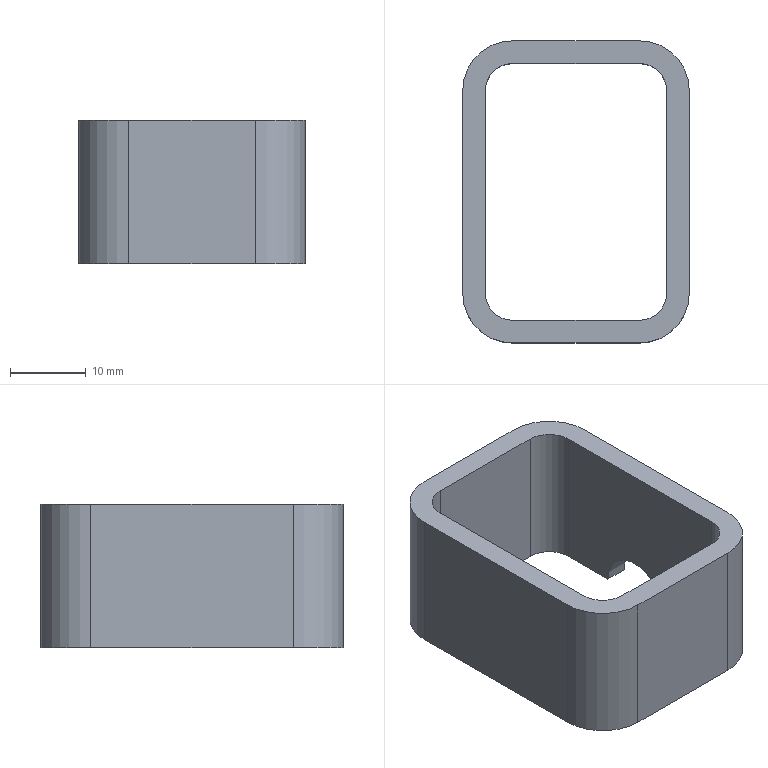Part | STEP file | DIN EN 10305-5 40 x 30 x 3 1785420022083 | 1 solid | 19 faces | box 30 x 40 x 19 mm | volume 6679 mm3 | plane 10 | cylinder 9 | commonest cylinder face diameters 7.2 x4 13.2 x4 10 x1
STEP:
#1=CARTESIAN_POINT('',(15.,-13.4,19.));
#2=VERTEX_POINT('',#1);
#3=CARTESIAN_POINT('',(8.4,-20.,19.));
#4=VERTEX_POINT('',#3);
#5=CARTESIAN_POINT('',(8.4,-13.4,19.));
#6=DIRECTION('',(0.,0.,-1.));
#7=DIRECTION('',(0.,1.,0.));
#8=AXIS2_PLACEMENT_3D('',#5,#6,#7);
#9=CIRCLE('',#8,6.6);
#10=EDGE_CURVE('',#2,#4,#9,.T.);
#11=ORIENTED_EDGE('',*,*,#10,.F.);
#12=CARTESIAN_POINT('',(15.,13.4,19.));
#13=VERTEX_POINT('',#12);
#14=CARTESIAN_POINT('',(15.,-48.3,19.));
#15=DIRECTION('',(0.,-1.,0.));
#16=VECTOR('',#15,10.);
#17=LINE('',#14,#16);
#18=EDGE_CURVE('',#13,#2,#17,.T.);
#19=ORIENTED_EDGE('',*,*,#18,.F.);
#20=CARTESIAN_POINT('',(8.4,20.,19.));
#21=VERTEX_POINT('',#20);
#22=CARTESIAN_POINT('',(8.4,13.4,19.));
#23=DIRECTION('',(0.,0.,-1.));
#24=DIRECTION('',(-1.,0.,0.));
#25=AXIS2_PLACEMENT_3D('',#22,#23,#24);
#26=CIRCLE('',#25,6.6);
#27=EDGE_CURVE('',#21,#13,#26,.T.);
#28=ORIENTED_EDGE('',*,*,#27,.F.);
#29=CARTESIAN_POINT('',(-8.4,20.,19.));
#30=VERTEX_POINT('',#29);
#31=CARTESIAN_POINT('',(-4.2,20.,19.));
#32=DIRECTION('',(1.,0.,0.));
#33=VECTOR('',#32,10.);
#34=LINE('',#31,#33);
#35=EDGE_CURVE('',#30,#21,#34,.T.);
#36=ORIENTED_EDGE('',*,*,#35,.F.);
#37=CARTESIAN_POINT('',(-15.,13.4,19.));
#38=VERTEX_POINT('',#37);
#39=CARTESIAN_POINT('',(-8.4,13.4,19.));
#40=DIRECTION('',(0.,0.,-1.));
#41=DIRECTION('',(0.,-1.,0.));
#42=AXIS2_PLACEMENT_3D('',#39,#40,#41);
#43=CIRCLE('',#42,6.6);
#44=EDGE_CURVE('',#38,#30,#43,.T.);
#45=ORIENTED_EDGE('',*,*,#44,.F.);
#46=CARTESIAN_POINT('',(-15.,-13.4,19.));
#47=VERTEX_POINT('',#46);
#48=CARTESIAN_POINT('',(-15.,-61.7,19.));
#49=DIRECTION('',(0.,1.,0.));
#50=VECTOR('',#49,10.);
#51=LINE('',#48,#50);
#52=EDGE_CURVE('',#47,#38,#51,.T.);
#53=ORIENTED_EDGE('',*,*,#52,.F.);
#54=CARTESIAN_POINT('',(-8.4,-20.,19.));
#55=VERTEX_POINT('',#54);
#56=CARTESIAN_POINT('',(-8.4,-13.4,19.));
#57=DIRECTION('',(0.,0.,-1.));
#58=DIRECTION('',(1.,0.,0.));
#59=AXIS2_PLACEMENT_3D('',#56,#57,#58);
#60=CIRCLE('',#59,6.6);
#61=EDGE_CURVE('',#55,#47,#60,.T.);
#62=ORIENTED_EDGE('',*,*,#61,.F.);
#63=CARTESIAN_POINT('',(4.2,-20.,19.));
#64=DIRECTION('',(-1.,0.,0.));
#65=VECTOR('',#64,10.);
#66=LINE('',#63,#65);
#67=EDGE_CURVE('',#4,#55,#66,.T.);
#68=ORIENTED_EDGE('',*,*,#67,.F.);
#69=EDGE_LOOP('',(#11,#19,#28,#36,#45,#53,#62,#68));
#70=FACE_OUTER_BOUND('',#69,.T.);
#71=CARTESIAN_POINT('',(12.,-13.4,19.));
#72=VERTEX_POINT('',#71);
#73=CARTESIAN_POINT('',(12.,13.4,19.));
#74=VERTEX_POINT('',#73);
#75=CARTESIAN_POINT('',(12.,-48.3,19.));
#76=DIRECTION('',(0.,1.,0.));
#77=VECTOR('',#76,10.);
#78=LINE('',#75,#77);
#79=EDGE_CURVE('',#72,#74,#78,.T.);
#80=ORIENTED_EDGE('',*,*,#79,.F.);
#81=CARTESIAN_POINT('',(8.4,-17.,19.));
#82=VERTEX_POINT('',#81);
#83=CARTESIAN_POINT('',(8.4,-13.4,19.));
#84=DIRECTION('',(0.,0.,1.));
#85=DIRECTION('',(0.,1.,0.));
#86=AXIS2_PLACEMENT_3D('',#83,#84,#85);
#87=CIRCLE('',#86,3.6);
#88=EDGE_CURVE('',#82,#72,#87,.T.);
#89=ORIENTED_EDGE('',*,*,#88,.F.);
#90=CARTESIAN_POINT('',(-8.4,-17.,19.));
#91=VERTEX_POINT('',#90);
#92=CARTESIAN_POINT('',(4.2,-17.,19.));
#93=DIRECTION('',(1.,0.,0.));
#94=VECTOR('',#93,10.);
#95=LINE('',#92,#94);
#96=EDGE_CURVE('',#91,#82,#95,.T.);
#97=ORIENTED_EDGE('',*,*,#96,.F.);
#98=CARTESIAN_POINT('',(-12.,-13.4,19.));
#99=VERTEX_POINT('',#98);
#100=CARTESIAN_POINT('',(-8.4,-13.4,19.));
#101=DIRECTION('',(0.,0.,1.));
#102=DIRECTION('',(1.,0.,0.));
#103=AXIS2_PLACEMENT_3D('',#100,#101,#102);
#104=CIRCLE('',#103,3.6);
#105=EDGE_CURVE('',#99,#91,#104,.T.);
#106=ORIENTED_EDGE('',*,*,#105,.F.);
#107=CARTESIAN_POINT('',(-12.,13.4,19.));
#108=VERTEX_POINT('',#107);
#109=CARTESIAN_POINT('',(-12.,-61.7,19.));
#110=DIRECTION('',(0.,-1.,0.));
#111=VECTOR('',#110,10.);
#112=LINE('',#109,#111);
#113=EDGE_CURVE('',#108,#99,#112,.T.);
#114=ORIENTED_EDGE('',*,*,#113,.F.);
#115=CARTESIAN_POINT('',(-8.4,17.,19.));
#116=VERTEX_POINT('',#115);
#117=CARTESIAN_POINT('',(-8.4,13.4,19.));
#118=DIRECTION('',(0.,0.,1.));
#119=DIRECTION('',(0.,-1.,0.));
#120=AXIS2_PLACEMENT_3D('',#117,#118,#119);
#121=CIRCLE('',#120,3.6);
#122=EDGE_CURVE('',#116,#108,#121,.T.);
#123=ORIENTED_EDGE('',*,*,#122,.F.);
#124=CARTESIAN_POINT('',(8.4,17.,19.));
#125=VERTEX_POINT('',#124);
#126=CARTESIAN_POINT('',(-4.2,17.,19.));
#127=DIRECTION('',(-1.,0.,0.));
#128=VECTOR('',#127,10.);
#129=LINE('',#126,#128);
#130=EDGE_CURVE('',#125,#116,#129,.T.);
#131=ORIENTED_EDGE('',*,*,#130,.F.);
#132=CARTESIAN_POINT('',(8.4,13.4,19.));
#133=DIRECTION('',(0.,0.,1.));
#134=DIRECTION('',(-1.,0.,0.));
#135=AXIS2_PLACEMENT_3D('',#132,#133,#134);
#136=CIRCLE('',#135,3.6);
#137=EDGE_CURVE('',#74,#125,#136,.T.);
#138=ORIENTED_EDGE('',*,*,#137,.F.);
#139=EDGE_LOOP('',(#80,#89,#97,#106,#114,#123,#131,#138));
#140=FACE_BOUND('',#139,.T.);
#141=CARTESIAN_POINT('',(0.,-110.,19.));
#142=DIRECTION('',(0.,0.,1.));
#143=DIRECTION('',(-1.,0.,0.));
#144=AXIS2_PLACEMENT_3D('',#141,#142,#143);
#145=PLANE('',#144);
#146=ADVANCED_FACE('',(#70,#140),#145,.T.);
#147=ORIENTED_EDGE('',*,*,#137,.T.);
#148=CARTESIAN_POINT('',(8.4,17.,0.));
#149=VERTEX_POINT('',#148);
#150=CARTESIAN_POINT('',(8.4,17.,0.));
#151=DIRECTION('',(0.,0.,1.));
#152=VECTOR('',#151,10.);
#153=LINE('',#150,#152);
#154=EDGE_CURVE('',#149,#125,#153,.T.);
#155=ORIENTED_EDGE('',*,*,#154,.F.);
#156=CARTESIAN_POINT('',(12.,13.4,0.));
#157=VERTEX_POINT('',#156);
#158=CARTESIAN_POINT('',(8.4,13.4,0.));
#159=DIRECTION('',(0.,0.,1.));
#160=DIRECTION('',(-1.,0.,0.));
#161=AXIS2_PLACEMENT_3D('',#158,#159,#160);
#162=CIRCLE('',#161,3.6);
#163=EDGE_CURVE('',#157,#149,#162,.T.);
#164=ORIENTED_EDGE('',*,*,#163,.F.);
#165=CARTESIAN_POINT('',(12.,13.4,0.));
#166=DIRECTION('',(0.,0.,1.));
#167=VECTOR('',#166,10.);
#168=LINE('',#165,#167);
#169=EDGE_CURVE('',#157,#74,#168,.T.);
#170=ORIENTED_EDGE('',*,*,#169,.T.);
#171=EDGE_LOOP('',(#147,#155,#164,#170));
#172=FACE_OUTER_BOUND('',#171,.T.);
#173=CARTESIAN_POINT('',(8.4,13.4,0.));
#174=DIRECTION('',(0.,0.,1.));
#175=DIRECTION('',(-1.,0.,0.));
#176=AXIS2_PLACEMENT_3D('',#173,#174,#175);
#177=CYLINDRICAL_SURFACE('',#176,3.6);
#178=ADVANCED_FACE('',(#172),#177,.F.);
#179=ORIENTED_EDGE('',*,*,#130,.T.);
#180=CARTESIAN_POINT('',(-8.4,17.,0.));
#181=VERTEX_POINT('',#180);
#182=CARTESIAN_POINT('',(-8.4,17.,0.));
#183=DIRECTION('',(0.,0.,1.));
#184=VECTOR('',#183,10.);
#185=LINE('',#182,#184);
#186=EDGE_CURVE('',#181,#116,#185,.T.);
#187=ORIENTED_EDGE('',*,*,#186,.F.);
#188=CARTESIAN_POINT('',(-4.2,17.,0.));
#189=DIRECTION('',(-1.,0.,0.));
#190=VECTOR('',#189,10.);
#191=LINE('',#188,#190);
#192=EDGE_CURVE('',#149,#181,#191,.T.);
#193=ORIENTED_EDGE('',*,*,#192,.F.);
#194=ORIENTED_EDGE('',*,*,#154,.T.);
#195=EDGE_LOOP('',(#179,#187,#193,#194));
#196=FACE_OUTER_BOUND('',#195,.T.);
#197=CARTESIAN_POINT('',(-8.4,17.,0.));
#198=DIRECTION('',(0.,1.,0.));
#199=DIRECTION('',(0.,0.,1.));
#200=AXIS2_PLACEMENT_3D('',#197,#198,#199);
#201=PLANE('',#200);
#202=ADVANCED_FACE('',(#196),#201,.F.);
#203=ORIENTED_EDGE('',*,*,#122,.T.);
#204=CARTESIAN_POINT('',(-12.,13.4,0.));
#205=VERTEX_POINT('',#204);
#206=CARTESIAN_POINT('',(-12.,13.4,0.));
#207=DIRECTION('',(0.,0.,1.));
#208=VECTOR('',#207,10.);
#209=LINE('',#206,#208);
#210=EDGE_CURVE('',#205,#108,#209,.T.);
#211=ORIENTED_EDGE('',*,*,#210,.F.);
#212=CARTESIAN_POINT('',(-8.4,13.4,0.));
#213=DIRECTION('',(0.,0.,1.));
#214=DIRECTION('',(0.,-1.,0.));
#215=AXIS2_PLACEMENT_3D('',#212,#213,#214);
#216=CIRCLE('',#215,3.6);
#217=EDGE_CURVE('',#181,#205,#216,.T.);
#218=ORIENTED_EDGE('',*,*,#217,.F.);
#219=ORIENTED_EDGE('',*,*,#186,.T.);
#220=EDGE_LOOP('',(#203,#211,#218,#219));
#221=FACE_OUTER_BOUND('',#220,.T.);
#222=CARTESIAN_POINT('',(-8.4,13.4,0.));
#223=DIRECTION('',(0.,0.,1.));
#224=DIRECTION('',(0.,-1.,0.));
#225=AXIS2_PLACEMENT_3D('',#222,#223,#224);
#226=CYLINDRICAL_SURFACE('',#225,3.6);
#227=ADVANCED_FACE('',(#221),#226,.F.);
#228=ORIENTED_EDGE('',*,*,#113,.T.);
#229=CARTESIAN_POINT('',(-12.,-13.4,0.));
#230=VERTEX_POINT('',#229);
#231=CARTESIAN_POINT('',(-12.,-13.4,0.));
#232=DIRECTION('',(0.,0.,1.));
#233=VECTOR('',#232,10.);
#234=LINE('',#231,#233);
#235=EDGE_CURVE('',#230,#99,#234,.T.);
#236=ORIENTED_EDGE('',*,*,#235,.F.);
#237=CARTESIAN_POINT('',(-12.,-6.7,0.));
#238=DIRECTION('',(0.,-1.,0.));
#239=VECTOR('',#238,10.);
#240=LINE('',#237,#239);
#241=EDGE_CURVE('',#205,#230,#240,.T.);
#242=ORIENTED_EDGE('',*,*,#241,.F.);
#243=ORIENTED_EDGE('',*,*,#210,.T.);
#244=EDGE_LOOP('',(#228,#236,#242,#243));
#245=FACE_OUTER_BOUND('',#244,.T.);
#246=CARTESIAN_POINT('',(-12.,-13.4,0.));
#247=DIRECTION('',(-1.,0.,0.));
#248=DIRECTION('',(0.,0.,1.));
#249=AXIS2_PLACEMENT_3D('',#246,#247,#248);
#250=PLANE('',#249);
#251=ADVANCED_FACE('',(#245),#250,.F.);
#252=ORIENTED_EDGE('',*,*,#67,.T.);
#253=CARTESIAN_POINT('',(-8.4,-20.,0.));
#254=VERTEX_POINT('',#253);
#255=CARTESIAN_POINT('',(-8.4,-20.,0.));
#256=DIRECTION('',(0.,0.,1.));
#257=VECTOR('',#256,10.);
#258=LINE('',#255,#257);
#259=EDGE_CURVE('',#254,#55,#258,.T.);
#260=ORIENTED_EDGE('',*,*,#259,.F.);
#261=CARTESIAN_POINT('',(8.4,-20.,0.));
#262=VERTEX_POINT('',#261);
#263=CARTESIAN_POINT('',(4.2,-20.,0.));
#264=DIRECTION('',(-1.,0.,0.));
#265=VECTOR('',#264,10.);
#266=LINE('',#263,#265);
#267=EDGE_CURVE('',#262,#254,#266,.T.);
#268=ORIENTED_EDGE('',*,*,#267,.F.);
#269=CARTESIAN_POINT('',(8.4,-20.,0.));
#270=DIRECTION('',(0.,0.,1.));
#271=VECTOR('',#270,10.);
#272=LINE('',#269,#271);
#273=EDGE_CURVE('',#262,#4,#272,.T.);
#274=ORIENTED_EDGE('',*,*,#273,.T.);
#275=EDGE_LOOP('',(#252,#260,#268,#274));
#276=FACE_OUTER_BOUND('',#275,.T.);
#277=CARTESIAN_POINT('',(8.4,-20.,0.));
#278=DIRECTION('',(0.,-1.,0.));
#279=DIRECTION('',(0.,0.,-1.));
#280=AXIS2_PLACEMENT_3D('',#277,#278,#279);
#281=PLANE('',#280);
#282=ADVANCED_FACE('',(#276),#281,.T.);
#283=ORIENTED_EDGE('',*,*,#61,.T.);
#284=CARTESIAN_POINT('',(-15.,-13.4,0.));
#285=VERTEX_POINT('',#284);
#286=CARTESIAN_POINT('',(-15.,-13.4,0.));
#287=DIRECTION('',(0.,0.,1.));
#288=VECTOR('',#287,10.);
#289=LINE('',#286,#288);
#290=EDGE_CURVE('',#285,#47,#289,.T.);
#291=ORIENTED_EDGE('',*,*,#290,.F.);
#292=CARTESIAN_POINT('',(-8.4,-13.4,0.));
#293=DIRECTION('',(0.,0.,-1.));
#294=DIRECTION('',(1.,0.,0.));
#295=AXIS2_PLACEMENT_3D('',#292,#293,#294);
#296=CIRCLE('',#295,6.6);
#297=EDGE_CURVE('',#254,#285,#296,.T.);
#298=ORIENTED_EDGE('',*,*,#297,.F.);
#299=ORIENTED_EDGE('',*,*,#259,.T.);
#300=EDGE_LOOP('',(#283,#291,#298,#299));
#301=FACE_OUTER_BOUND('',#300,.T.);
#302=CARTESIAN_POINT('',(-8.4,-13.4,0.));
#303=DIRECTION('',(0.,0.,1.));
#304=DIRECTION('',(1.,0.,0.));
#305=AXIS2_PLACEMENT_3D('',#302,#303,#304);
#306=CYLINDRICAL_SURFACE('',#305,6.6);
#307=ADVANCED_FACE('',(#301),#306,.T.);
#308=ORIENTED_EDGE('',*,*,#52,.T.);
#309=CARTESIAN_POINT('',(-15.,13.4,0.));
#310=VERTEX_POINT('',#309);
#311=CARTESIAN_POINT('',(-15.,13.4,0.));
#312=DIRECTION('',(0.,0.,1.));
#313=VECTOR('',#312,10.);
#314=LINE('',#311,#313);
#315=EDGE_CURVE('',#310,#38,#314,.T.);
#316=ORIENTED_EDGE('',*,*,#315,.F.);
#317=CARTESIAN_POINT('',(-15.,-6.7,0.));
#318=DIRECTION('',(0.,1.,0.));
#319=VECTOR('',#318,10.);
#320=LINE('',#317,#319);
#321=EDGE_CURVE('',#285,#310,#320,.T.);
#322=ORIENTED_EDGE('',*,*,#321,.F.);
#323=ORIENTED_EDGE('',*,*,#290,.T.);
#324=EDGE_LOOP('',(#308,#316,#322,#323));
#325=FACE_OUTER_BOUND('',#324,.T.);
#326=CARTESIAN_POINT('',(-15.,-13.4,0.));
#327=DIRECTION('',(-1.,0.,0.));
#328=DIRECTION('',(0.,0.,1.));
#329=AXIS2_PLACEMENT_3D('',#326,#327,#328);
#330=PLANE('',#329);
#331=ADVANCED_FACE('',(#325),#330,.T.);
#332=ORIENTED_EDGE('',*,*,#44,.T.);
#333=CARTESIAN_POINT('',(-8.4,20.,0.));
#334=VERTEX_POINT('',#333);
#335=CARTESIAN_POINT('',(-8.4,20.,0.));
#336=DIRECTION('',(0.,0.,1.));
#337=VECTOR('',#336,10.);
#338=LINE('',#335,#337);
#339=EDGE_CURVE('',#334,#30,#338,.T.);
#340=ORIENTED_EDGE('',*,*,#339,.F.);
#341=CARTESIAN_POINT('',(-8.4,13.4,0.));
#342=DIRECTION('',(0.,0.,-1.));
#343=DIRECTION('',(0.,-1.,0.));
#344=AXIS2_PLACEMENT_3D('',#341,#342,#343);
#345=CIRCLE('',#344,6.6);
#346=EDGE_CURVE('',#310,#334,#345,.T.);
#347=ORIENTED_EDGE('',*,*,#346,.F.);
#348=ORIENTED_EDGE('',*,*,#315,.T.);
#349=EDGE_LOOP('',(#332,#340,#347,#348));
#350=FACE_OUTER_BOUND('',#349,.T.);
#351=CARTESIAN_POINT('',(-8.4,13.4,0.));
#352=DIRECTION('',(0.,0.,1.));
#353=DIRECTION('',(0.,-1.,0.));
#354=AXIS2_PLACEMENT_3D('',#351,#352,#353);
#355=CYLINDRICAL_SURFACE('',#354,6.6);
#356=ADVANCED_FACE('',(#350),#355,.T.);
#357=CARTESIAN_POINT('',(15.,6.012,0.));
#358=VERTEX_POINT('',#357);
#359=CARTESIAN_POINT('',(12.,6.012,0.));
#360=VERTEX_POINT('',#359);
#361=CARTESIAN_POINT('',(15.,6.012,0.));
#362=DIRECTION('',(-1.,0.,0.));
#363=VECTOR('',#362,10.);
#364=LINE('',#361,#363);
#365=EDGE_CURVE('',#358,#360,#364,.T.);
#366=ORIENTED_EDGE('',*,*,#365,.F.);
#367=CARTESIAN_POINT('',(15.,-3.988,0.));
#368=VERTEX_POINT('',#367);
#369=CARTESIAN_POINT('',(15.,1.012,0.));
#370=DIRECTION('',(-1.,0.,0.));
#371=DIRECTION('',(0.,0.,-1.));
#372=AXIS2_PLACEMENT_3D('',#369,#370,#371);
#373=CIRCLE('',#372,5.);
#374=EDGE_CURVE('',#368,#358,#373,.T.);
#375=ORIENTED_EDGE('',*,*,#374,.F.);
#376=CARTESIAN_POINT('',(12.,-3.988,0.));
#377=VERTEX_POINT('',#376);
#378=CARTESIAN_POINT('',(15.,-3.988,0.));
#379=DIRECTION('',(1.,0.,0.));
#380=VECTOR('',#379,10.);
#381=LINE('',#378,#380);
#382=EDGE_CURVE('',#377,#368,#381,.T.);
#383=ORIENTED_EDGE('',*,*,#382,.F.);
#384=CARTESIAN_POINT('',(12.,1.012,0.));
#385=DIRECTION('',(1.,0.,0.));
#386=DIRECTION('',(0.,0.,-1.));
#387=AXIS2_PLACEMENT_3D('',#384,#385,#386);
#388=CIRCLE('',#387,5.);
#389=EDGE_CURVE('',#360,#377,#388,.T.);
#390=ORIENTED_EDGE('',*,*,#389,.F.);
#391=EDGE_LOOP('',(#366,#375,#383,#390));
#392=FACE_OUTER_BOUND('',#391,.T.);
#393=CARTESIAN_POINT('',(15.,1.012,0.));
#394=DIRECTION('',(-1.,0.,0.));
#395=DIRECTION('',(0.,0.,1.));
#396=AXIS2_PLACEMENT_3D('',#393,#394,#395);
#397=CYLINDRICAL_SURFACE('',#396,5.);
#398=ADVANCED_FACE('',(#392),#397,.F.);
#399=ORIENTED_EDGE('',*,*,#79,.T.);
#400=ORIENTED_EDGE('',*,*,#169,.F.);
#401=CARTESIAN_POINT('',(12.,6.7,0.));
#402=DIRECTION('',(0.,1.,0.));
#403=VECTOR('',#402,10.);
#404=LINE('',#401,#403);
#405=EDGE_CURVE('',#360,#157,#404,.T.);
#406=ORIENTED_EDGE('',*,*,#405,.F.);
#407=ORIENTED_EDGE('',*,*,#389,.T.);
#408=CARTESIAN_POINT('',(12.,-13.4,0.));
#409=VERTEX_POINT('',#408);
#410=CARTESIAN_POINT('',(12.,6.7,0.));
#411=DIRECTION('',(0.,1.,0.));
#412=VECTOR('',#411,10.);
#413=LINE('',#410,#412);
#414=EDGE_CURVE('',#409,#377,#413,.T.);
#415=ORIENTED_EDGE('',*,*,#414,.F.);
#416=CARTESIAN_POINT('',(12.,-13.4,0.));
#417=DIRECTION('',(0.,0.,1.));
#418=VECTOR('',#417,10.);
#419=LINE('',#416,#418);
#420=EDGE_CURVE('',#409,#72,#419,.T.);
#421=ORIENTED_EDGE('',*,*,#420,.T.);
#422=EDGE_LOOP('',(#399,#400,#406,#407,#415,#421));
#423=FACE_OUTER_BOUND('',#422,.T.);
#424=CARTESIAN_POINT('',(12.,13.4,0.));
#425=DIRECTION('',(1.,0.,0.));
#426=DIRECTION('',(0.,0.,-1.));
#427=AXIS2_PLACEMENT_3D('',#424,#425,#426);
#428=PLANE('',#427);
#429=ADVANCED_FACE('',(#423),#428,.F.);
#430=ORIENTED_EDGE('',*,*,#96,.T.);
#431=CARTESIAN_POINT('',(8.4,-17.,0.));
#432=VERTEX_POINT('',#431);
#433=CARTESIAN_POINT('',(8.4,-17.,0.));
#434=DIRECTION('',(0.,0.,1.));
#435=VECTOR('',#434,10.);
#436=LINE('',#433,#435);
#437=EDGE_CURVE('',#432,#82,#436,.T.);
#438=ORIENTED_EDGE('',*,*,#437,.F.);
#439=CARTESIAN_POINT('',(-8.4,-17.,0.));
#440=VERTEX_POINT('',#439);
#441=CARTESIAN_POINT('',(4.2,-17.,0.));
#442=DIRECTION('',(1.,0.,0.));
#443=VECTOR('',#442,10.);
#444=LINE('',#441,#443);
#445=EDGE_CURVE('',#440,#432,#444,.T.);
#446=ORIENTED_EDGE('',*,*,#445,.F.);
#447=CARTESIAN_POINT('',(-8.4,-17.,0.));
#448=DIRECTION('',(0.,0.,1.));
#449=VECTOR('',#448,10.);
#450=LINE('',#447,#449);
#451=EDGE_CURVE('',#440,#91,#450,.T.);
#452=ORIENTED_EDGE('',*,*,#451,.T.);
#453=EDGE_LOOP('',(#430,#438,#446,#452));
#454=FACE_OUTER_BOUND('',#453,.T.);
#455=CARTESIAN_POINT('',(8.4,-17.,0.));
#456=DIRECTION('',(0.,-1.,0.));
#457=DIRECTION('',(0.,0.,-1.));
#458=AXIS2_PLACEMENT_3D('',#455,#456,#457);
#459=PLANE('',#458);
#460=ADVANCED_FACE('',(#454),#459,.F.);
#461=ORIENTED_EDGE('',*,*,#88,.T.);
#462=ORIENTED_EDGE('',*,*,#420,.F.);
#463=CARTESIAN_POINT('',(8.4,-13.4,0.));
#464=DIRECTION('',(0.,0.,1.));
#465=DIRECTION('',(0.,1.,0.));
#466=AXIS2_PLACEMENT_3D('',#463,#464,#465);
#467=CIRCLE('',#466,3.6);
#468=EDGE_CURVE('',#432,#409,#467,.T.);
#469=ORIENTED_EDGE('',*,*,#468,.F.);
#470=ORIENTED_EDGE('',*,*,#437,.T.);
#471=EDGE_LOOP('',(#461,#462,#469,#470));
#472=FACE_OUTER_BOUND('',#471,.T.);
#473=CARTESIAN_POINT('',(8.4,-13.4,0.));
#474=DIRECTION('',(0.,0.,1.));
#475=DIRECTION('',(0.,1.,0.));
#476=AXIS2_PLACEMENT_3D('',#473,#474,#475);
#477=CYLINDRICAL_SURFACE('',#476,3.6);
#478=ADVANCED_FACE('',(#472),#477,.F.);
#479=ORIENTED_EDGE('',*,*,#18,.T.);
#480=CARTESIAN_POINT('',(15.,-13.4,0.));
#481=VERTEX_POINT('',#480);
#482=CARTESIAN_POINT('',(15.,-13.4,0.));
#483=DIRECTION('',(0.,0.,1.));
#484=VECTOR('',#483,10.);
#485=LINE('',#482,#484);
#486=EDGE_CURVE('',#481,#2,#485,.T.);
#487=ORIENTED_EDGE('',*,*,#486,.F.);
#488=CARTESIAN_POINT('',(15.,6.7,0.));
#489=DIRECTION('',(0.,-1.,0.));
#490=VECTOR('',#489,10.);
#491=LINE('',#488,#490);
#492=EDGE_CURVE('',#368,#481,#491,.T.);
#493=ORIENTED_EDGE('',*,*,#492,.F.);
#494=ORIENTED_EDGE('',*,*,#374,.T.);
#495=CARTESIAN_POINT('',(15.,13.4,0.));
#496=VERTEX_POINT('',#495);
#497=CARTESIAN_POINT('',(15.,6.7,0.));
#498=DIRECTION('',(0.,-1.,0.));
#499=VECTOR('',#498,10.);
#500=LINE('',#497,#499);
#501=EDGE_CURVE('',#496,#358,#500,.T.);
#502=ORIENTED_EDGE('',*,*,#501,.F.);
#503=CARTESIAN_POINT('',(15.,13.4,0.));
#504=DIRECTION('',(0.,0.,1.));
#505=VECTOR('',#504,10.);
#506=LINE('',#503,#505);
#507=EDGE_CURVE('',#496,#13,#506,.T.);
#508=ORIENTED_EDGE('',*,*,#507,.T.);
#509=EDGE_LOOP('',(#479,#487,#493,#494,#502,#508));
#510=FACE_OUTER_BOUND('',#509,.T.);
#511=CARTESIAN_POINT('',(15.,13.4,0.));
#512=DIRECTION('',(1.,0.,0.));
#513=DIRECTION('',(0.,0.,-1.));
#514=AXIS2_PLACEMENT_3D('',#511,#512,#513);
#515=PLANE('',#514);
#516=ADVANCED_FACE('',(#510),#515,.T.);
#517=ORIENTED_EDGE('',*,*,#10,.T.);
#518=ORIENTED_EDGE('',*,*,#273,.F.);
#519=CARTESIAN_POINT('',(8.4,-13.4,0.));
#520=DIRECTION('',(0.,0.,-1.));
#521=DIRECTION('',(0.,1.,0.));
#522=AXIS2_PLACEMENT_3D('',#519,#520,#521);
#523=CIRCLE('',#522,6.6);
#524=EDGE_CURVE('',#481,#262,#523,.T.);
#525=ORIENTED_EDGE('',*,*,#524,.F.);
#526=ORIENTED_EDGE('',*,*,#486,.T.);
#527=EDGE_LOOP('',(#517,#518,#525,#526));
#528=FACE_OUTER_BOUND('',#527,.T.);
#529=CARTESIAN_POINT('',(8.4,-13.4,0.));
#530=DIRECTION('',(0.,0.,1.));
#531=DIRECTION('',(0.,1.,0.));
#532=AXIS2_PLACEMENT_3D('',#529,#530,#531);
#533=CYLINDRICAL_SURFACE('',#532,6.6);
#534=ADVANCED_FACE('',(#528),#533,.T.);
#535=ORIENTED_EDGE('',*,*,#105,.T.);
#536=ORIENTED_EDGE('',*,*,#451,.F.);
#537=CARTESIAN_POINT('',(-8.4,-13.4,0.));
#538=DIRECTION('',(0.,0.,1.));
#539=DIRECTION('',(1.,0.,0.));
#540=AXIS2_PLACEMENT_3D('',#537,#538,#539);
#541=CIRCLE('',#540,3.6);
#542=EDGE_CURVE('',#230,#440,#541,.T.);
#543=ORIENTED_EDGE('',*,*,#542,.F.);
#544=ORIENTED_EDGE('',*,*,#235,.T.);
#545=EDGE_LOOP('',(#535,#536,#543,#544));
#546=FACE_OUTER_BOUND('',#545,.T.);
#547=CARTESIAN_POINT('',(-8.4,-13.4,0.));
#548=DIRECTION('',(0.,0.,1.));
#549=DIRECTION('',(1.,0.,0.));
#550=AXIS2_PLACEMENT_3D('',#547,#548,#549);
#551=CYLINDRICAL_SURFACE('',#550,3.6);
#552=ADVANCED_FACE('',(#546),#551,.F.);
#553=ORIENTED_EDGE('',*,*,#35,.T.);
#554=CARTESIAN_POINT('',(8.4,20.,0.));
#555=VERTEX_POINT('',#554);
#556=CARTESIAN_POINT('',(8.4,20.,0.));
#557=DIRECTION('',(0.,0.,1.));
#558=VECTOR('',#557,10.);
#559=LINE('',#556,#558);
#560=EDGE_CURVE('',#555,#21,#559,.T.);
#561=ORIENTED_EDGE('',*,*,#560,.F.);
#562=CARTESIAN_POINT('',(-4.2,20.,0.));
#563=DIRECTION('',(1.,0.,0.));
#564=VECTOR('',#563,10.);
#565=LINE('',#562,#564);
#566=EDGE_CURVE('',#334,#555,#565,.T.);
#567=ORIENTED_EDGE('',*,*,#566,.F.);
#568=ORIENTED_EDGE('',*,*,#339,.T.);
#569=EDGE_LOOP('',(#553,#561,#567,#568));
#570=FACE_OUTER_BOUND('',#569,.T.);
#571=CARTESIAN_POINT('',(-8.4,20.,0.));
#572=DIRECTION('',(0.,1.,0.));
#573=DIRECTION('',(0.,0.,1.));
#574=AXIS2_PLACEMENT_3D('',#571,#572,#573);
#575=PLANE('',#574);
#576=ADVANCED_FACE('',(#570),#575,.T.);
#577=ORIENTED_EDGE('',*,*,#27,.T.);
#578=ORIENTED_EDGE('',*,*,#507,.F.);
#579=CARTESIAN_POINT('',(8.4,13.4,0.));
#580=DIRECTION('',(0.,0.,-1.));
#581=DIRECTION('',(-1.,0.,0.));
#582=AXIS2_PLACEMENT_3D('',#579,#580,#581);
#583=CIRCLE('',#582,6.6);
#584=EDGE_CURVE('',#555,#496,#583,.T.);
#585=ORIENTED_EDGE('',*,*,#584,.F.);
#586=ORIENTED_EDGE('',*,*,#560,.T.);
#587=EDGE_LOOP('',(#577,#578,#585,#586));
#588=FACE_OUTER_BOUND('',#587,.T.);
#589=CARTESIAN_POINT('',(8.4,13.4,0.));
#590=DIRECTION('',(0.,0.,1.));
#591=DIRECTION('',(-1.,0.,0.));
#592=AXIS2_PLACEMENT_3D('',#589,#590,#591);
#593=CYLINDRICAL_SURFACE('',#592,6.6);
#594=ADVANCED_FACE('',(#588),#593,.T.);
#595=ORIENTED_EDGE('',*,*,#365,.T.);
#596=ORIENTED_EDGE('',*,*,#405,.T.);
#597=ORIENTED_EDGE('',*,*,#163,.T.);
#598=ORIENTED_EDGE('',*,*,#192,.T.);
#599=ORIENTED_EDGE('',*,*,#217,.T.);
#600=ORIENTED_EDGE('',*,*,#241,.T.);
#601=ORIENTED_EDGE('',*,*,#542,.T.);
#602=ORIENTED_EDGE('',*,*,#445,.T.);
#603=ORIENTED_EDGE('',*,*,#468,.T.);
#604=ORIENTED_EDGE('',*,*,#414,.T.);
#605=ORIENTED_EDGE('',*,*,#382,.T.);
#606=ORIENTED_EDGE('',*,*,#492,.T.);
#607=ORIENTED_EDGE('',*,*,#524,.T.);
#608=ORIENTED_EDGE('',*,*,#267,.T.);
#609=ORIENTED_EDGE('',*,*,#297,.T.);
#610=ORIENTED_EDGE('',*,*,#321,.T.);
#611=ORIENTED_EDGE('',*,*,#346,.T.);
#612=ORIENTED_EDGE('',*,*,#566,.T.);
#613=ORIENTED_EDGE('',*,*,#584,.T.);
#614=ORIENTED_EDGE('',*,*,#501,.T.);
#615=EDGE_LOOP('',(#595,#596,#597,#598,#599,#600,#601,#602,#603,#604,#605,#606,#607,#608,#609,#610,#611,#612,#613,#614));
#616=FACE_OUTER_BOUND('',#615,.T.);
#617=CARTESIAN_POINT('',(0.,0.,0.));
#618=DIRECTION('',(0.,0.,1.));
#619=DIRECTION('',(1.,0.,0.));
#620=AXIS2_PLACEMENT_3D('',#617,#618,#619);
#621=PLANE('',#620);
#622=ADVANCED_FACE('',(#616),#621,.F.);
#623=CLOSED_SHELL('',(#146,#178,#202,#227,#251,#282,#307,#331,#356,#398,#429,#460,#478,#516,#534,#552,#576,#594,#622));
#624=MANIFOLD_SOLID_BREP('',#623);
#625=(LENGTH_UNIT()NAMED_UNIT(*)SI_UNIT(.MILLI.,.METRE.));
#626=UNCERTAINTY_MEASURE_WITH_UNIT(LENGTH_MEASURE(0.01),#625,'','');
#627=(NAMED_UNIT(*)PLANE_ANGLE_UNIT()SI_UNIT($,.RADIAN.));
#628=(NAMED_UNIT(*)SI_UNIT($,.STERADIAN.)SOLID_ANGLE_UNIT());
#629=(GEOMETRIC_REPRESENTATION_CONTEXT(3)GLOBAL_UNCERTAINTY_ASSIGNED_CONTEXT((#626))GLOBAL_UNIT_ASSIGNED_CONTEXT((#625,#627,#628))REPRESENTATION_CONTEXT('',''));
#630=ADVANCED_BREP_SHAPE_REPRESENTATION('',(#624),#629);